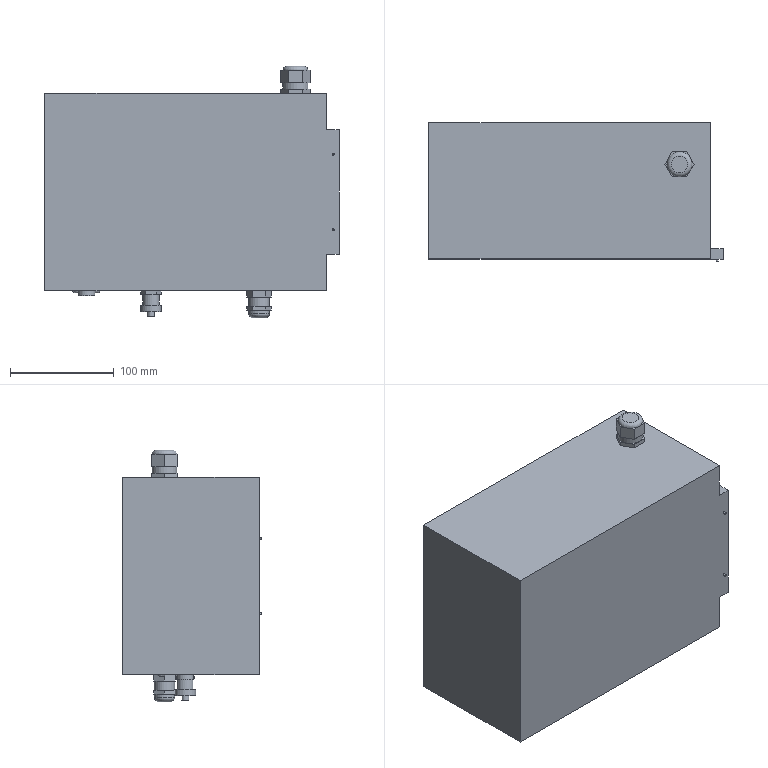Part | STEP file | a-hp_225_37-140_3_0_10 | 1 solid | 255 faces | box 283 x 133 x 242 mm | volume 6782742 mm3 | plane 184 | spline 58 | cylinder 11 | torus 2 | commonest cylinder face diameters 20 x4 2 x2 16 x2 7 x1 24 x1 30.5 x1